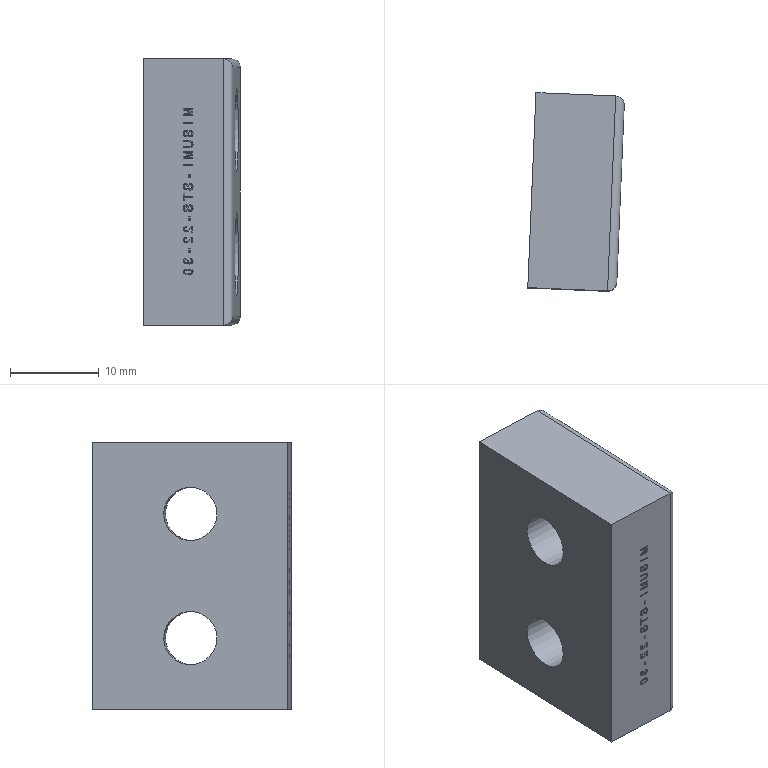Part | NX | features DB 2 | 1 solid | 307 faces | box 10.871 x 22.358 x 30 mm | volume 5544 mm3 | spline 210 | plane 89 | cylinder 8 | commonest cylinder face diameters 2 x4 6 x2 9.5 x2